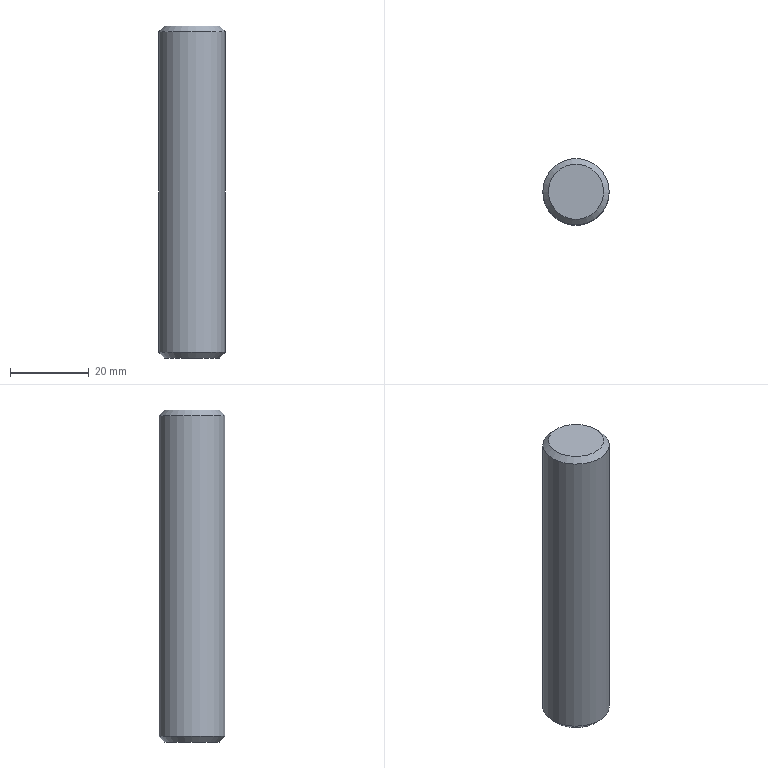Part | NX | features LINKED_BODY 2, DATUM_CSYS 1, Delete Body 1 | 1 solid | 5 faces | box 16.875 x 16.875 x 84.375 mm | volume 18772 mm3 | plane 2 | cone 2 | cylinder 1 | commonest cylinder face diameters 16.875 x1
STEP:
#1=CARTESIAN_POINT('',(-126.562,3441.692,-609.616));
#2=VERTEX_POINT('',#1);
#3=CARTESIAN_POINT('',(-118.125,3441.692,-609.616));
#4=DIRECTION('',(0.,0.,-1.));
#5=DIRECTION('',(-1.,0.,0.));
#6=AXIS2_PLACEMENT_3D('',#3,#4,#5);
#7=CIRCLE('',#6,8.438);
#8=EDGE_CURVE('',#2,#2,#7,.F.);
#9=ORIENTED_EDGE('',*,*,#8,.T.);
#10=EDGE_LOOP('',(#9));
#11=FACE_BOUND('',#10,.T.);
#12=CARTESIAN_POINT('',(-126.562,3441.692,-528.054));
#13=VERTEX_POINT('',#12);
#14=CARTESIAN_POINT('',(-118.125,3441.692,-528.054));
#15=DIRECTION('',(0.,0.,-1.));
#16=DIRECTION('',(-1.,0.,0.));
#17=AXIS2_PLACEMENT_3D('',#14,#15,#16);
#18=CIRCLE('',#17,8.438);
#19=EDGE_CURVE('',#13,#13,#18,.T.);
#20=ORIENTED_EDGE('',*,*,#19,.T.);
#21=EDGE_LOOP('',(#20));
#22=FACE_BOUND('',#21,.T.);
#23=CARTESIAN_POINT('',(-118.125,3441.692,-611.022));
#24=DIRECTION('',(0.,0.,1.));
#25=DIRECTION('',(1.,0.,0.));
#26=AXIS2_PLACEMENT_3D('',#23,#24,#25);
#27=CYLINDRICAL_SURFACE('',#26,8.438);
#28=ADVANCED_FACE('',(#11,#22),#27,.T.);
#29=CARTESIAN_POINT('',(-125.156,3441.692,-611.022));
#30=VERTEX_POINT('',#29);
#31=CARTESIAN_POINT('',(-118.125,3441.692,-611.022));
#32=DIRECTION('',(0.,0.,-1.));
#33=DIRECTION('',(-1.,0.,0.));
#34=AXIS2_PLACEMENT_3D('',#31,#32,#33);
#35=CIRCLE('',#34,7.031);
#36=EDGE_CURVE('',#30,#30,#35,.T.);
#37=ORIENTED_EDGE('',*,*,#36,.T.);
#38=EDGE_LOOP('',(#37));
#39=FACE_BOUND('',#38,.T.);
#40=CARTESIAN_POINT('',(-118.125,3441.692,-611.022));
#41=DIRECTION('',(0.,0.,-1.));
#42=DIRECTION('',(-1.,0.,0.));
#43=AXIS2_PLACEMENT_3D('',#40,#41,#42);
#44=PLANE('',#43);
#45=ADVANCED_FACE('',(#39),#44,.T.);
#46=CARTESIAN_POINT('',(-125.156,3441.692,-526.647));
#47=VERTEX_POINT('',#46);
#48=CARTESIAN_POINT('',(-118.125,3441.692,-526.647));
#49=DIRECTION('',(0.,0.,-1.));
#50=DIRECTION('',(-1.,0.,0.));
#51=AXIS2_PLACEMENT_3D('',#48,#49,#50);
#52=CIRCLE('',#51,7.031);
#53=EDGE_CURVE('',#47,#47,#52,.F.);
#54=ORIENTED_EDGE('',*,*,#53,.T.);
#55=EDGE_LOOP('',(#54));
#56=FACE_BOUND('',#55,.T.);
#57=CARTESIAN_POINT('',(-118.125,3441.692,-526.647));
#58=DIRECTION('',(0.,0.,-1.));
#59=DIRECTION('',(-1.,0.,0.));
#60=AXIS2_PLACEMENT_3D('',#57,#58,#59);
#61=PLANE('',#60);
#62=ADVANCED_FACE('',(#56),#61,.F.);
#63=ORIENTED_EDGE('',*,*,#8,.F.);
#64=EDGE_LOOP('',(#63));
#65=FACE_BOUND('',#64,.T.);
#66=ORIENTED_EDGE('',*,*,#36,.F.);
#67=EDGE_LOOP('',(#66));
#68=FACE_BOUND('',#67,.T.);
#69=CARTESIAN_POINT('',(-118.125,3441.692,-611.022));
#70=DIRECTION('',(0.,0.,1.));
#71=DIRECTION('',(1.,0.,0.));
#72=AXIS2_PLACEMENT_3D('',#69,#70,#71);
#73=CONICAL_SURFACE('',#72,7.031,0.7854);
#74=ADVANCED_FACE('',(#65,#68),#73,.T.);
#75=ORIENTED_EDGE('',*,*,#53,.F.);
#76=EDGE_LOOP('',(#75));
#77=FACE_BOUND('',#76,.T.);
#78=ORIENTED_EDGE('',*,*,#19,.F.);
#79=EDGE_LOOP('',(#78));
#80=FACE_BOUND('',#79,.T.);
#81=CARTESIAN_POINT('',(-118.125,3441.692,-528.054));
#82=DIRECTION('',(0.,0.,-1.));
#83=DIRECTION('',(-1.,0.,0.));
#84=AXIS2_PLACEMENT_3D('',#81,#82,#83);
#85=CONICAL_SURFACE('',#84,8.438,0.7854);
#86=ADVANCED_FACE('',(#77,#80),#85,.T.);
#87=CLOSED_SHELL('',(#28,#45,#62,#74,#86));
#88=MANIFOLD_SOLID_BREP('',#87);
#89=(LENGTH_UNIT()NAMED_UNIT(*)SI_UNIT(.MILLI.,.METRE.));
#90=UNCERTAINTY_MEASURE_WITH_UNIT(LENGTH_MEASURE(0.00001),#89,'','');
#91=(NAMED_UNIT(*)PLANE_ANGLE_UNIT()SI_UNIT($,.RADIAN.));
#92=(NAMED_UNIT(*)SI_UNIT($,.STERADIAN.)SOLID_ANGLE_UNIT());
#93=(GEOMETRIC_REPRESENTATION_CONTEXT(3)GLOBAL_UNCERTAINTY_ASSIGNED_CONTEXT((#90))GLOBAL_UNIT_ASSIGNED_CONTEXT((#89,#91,#92))REPRESENTATION_CONTEXT('',''));
#94=ADVANCED_BREP_SHAPE_REPRESENTATION('',(#88),#93);